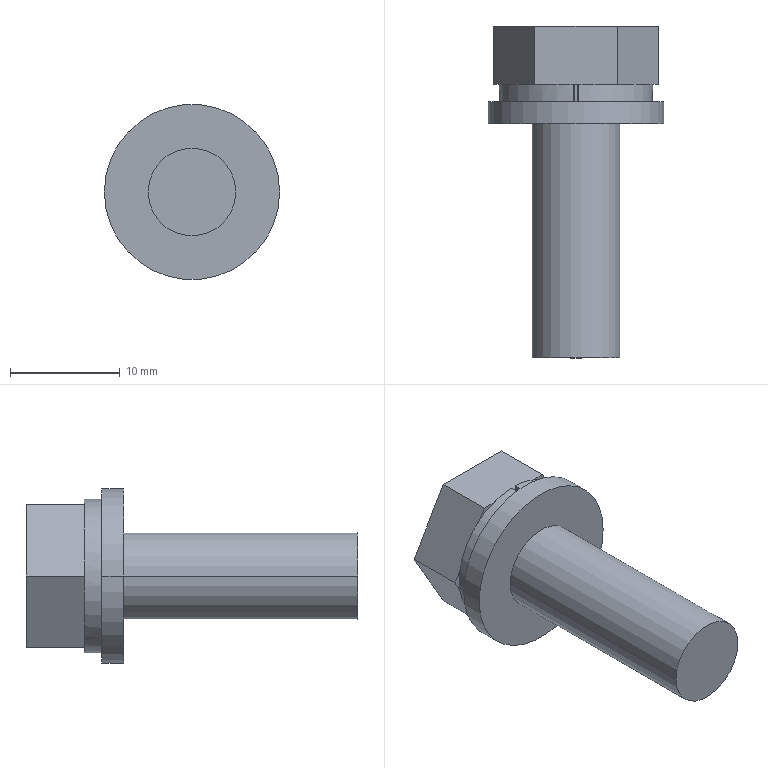Part | STEP file | LIB_36623179_M8X25 | 1 solid | 32 faces | box 16 x 30.3 x 16 mm | volume 2498 mm3 | plane 26 | cylinder 6 | commonest cylinder face diameters 8 x3 16 x2 14 x1